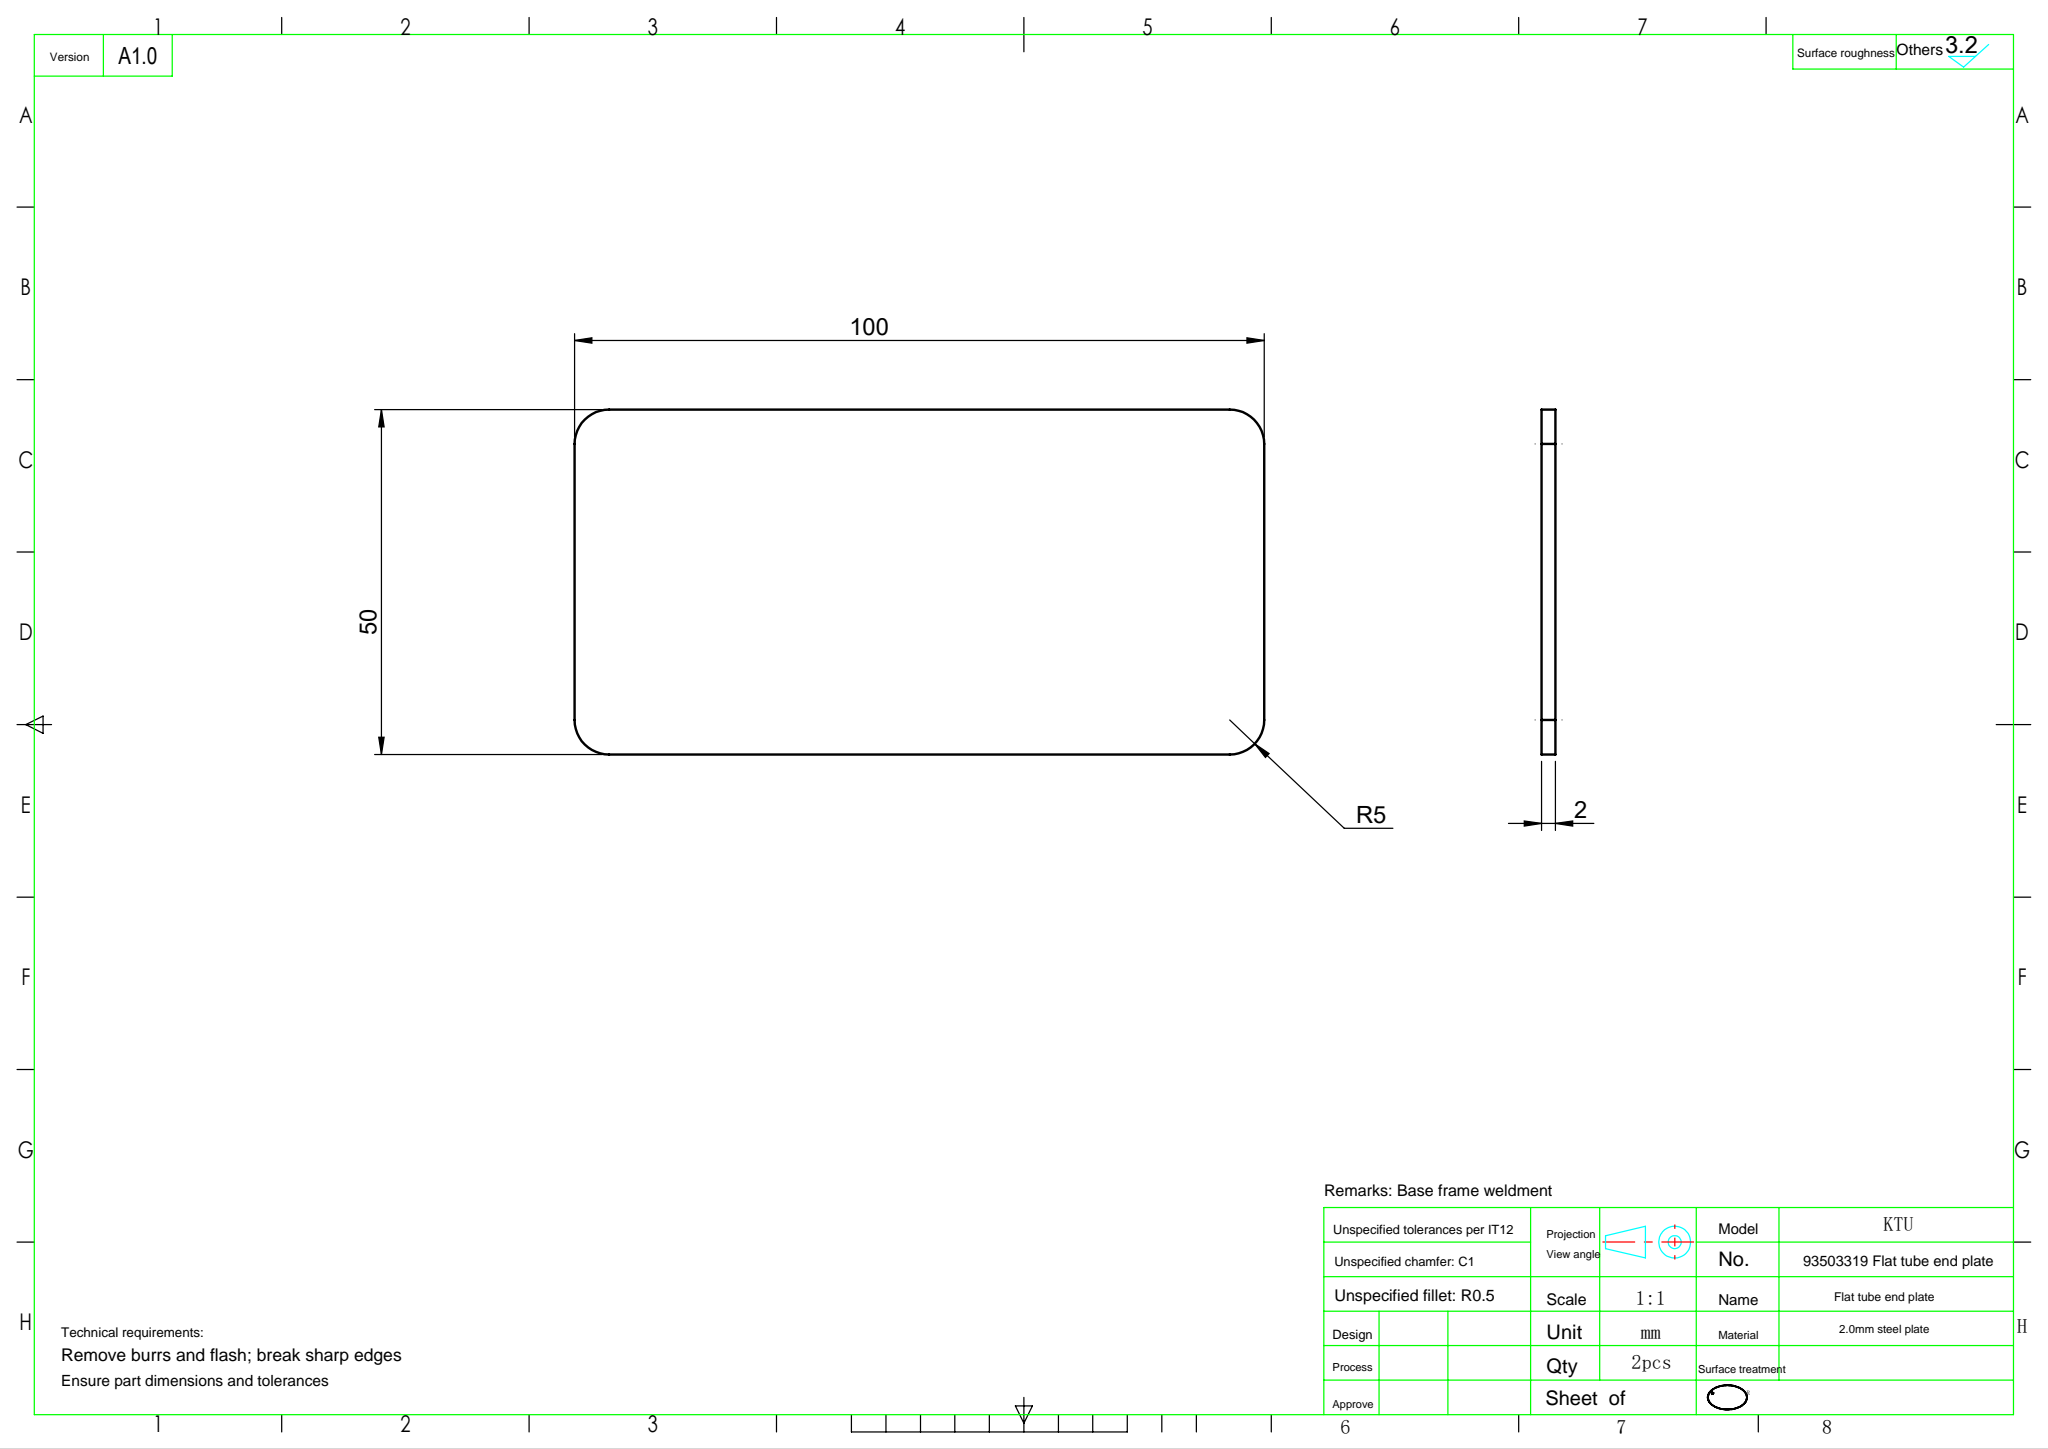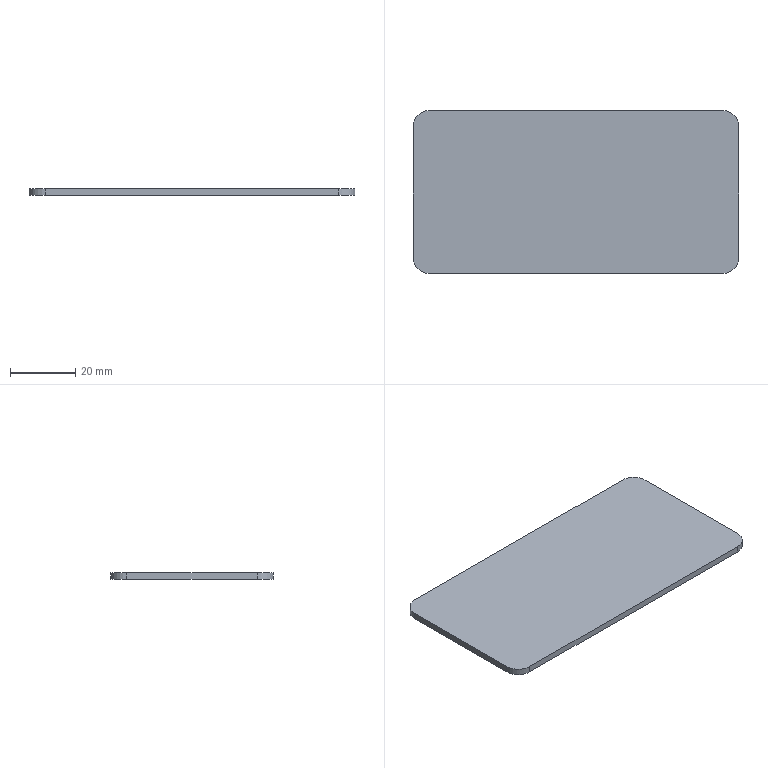Part | SolidWorks | features FlatPattern 1, SMBaseFlange 1, SheetMetal 1 | 1 solid | 10 faces | box 100 x 50 x 2 mm | volume 9957 mm3 | plane 6 | cylinder 4 | commonest cylinder face diameters 10 x4
STEP:
#1=CARTESIAN_POINT('',(45.,-25.,0.));
#2=VERTEX_POINT('',#1);
#3=CARTESIAN_POINT('',(50.,-20.,0.));
#4=VERTEX_POINT('',#3);
#5=CARTESIAN_POINT('',(45.,-20.,0.));
#6=DIRECTION('',(0.,0.,1.));
#7=DIRECTION('',(1.,0.,0.));
#8=AXIS2_PLACEMENT_3D('',#5,#6,#7);
#9=CIRCLE('',#8,5.);
#10=EDGE_CURVE('',#2,#4,#9,.T.);
#11=ORIENTED_EDGE('',*,*,#10,.F.);
#12=CARTESIAN_POINT('',(45.,-25.,-2.));
#13=VERTEX_POINT('',#12);
#14=CARTESIAN_POINT('',(45.,-25.,-2.));
#15=DIRECTION('',(0.,0.,1.));
#16=VECTOR('',#15,1000.);
#17=LINE('',#14,#16);
#18=EDGE_CURVE('',#13,#2,#17,.T.);
#19=ORIENTED_EDGE('',*,*,#18,.F.);
#20=CARTESIAN_POINT('',(50.,-20.,-2.));
#21=VERTEX_POINT('',#20);
#22=CARTESIAN_POINT('',(45.,-20.,-2.));
#23=DIRECTION('',(0.,0.,1.));
#24=DIRECTION('',(1.,0.,0.));
#25=AXIS2_PLACEMENT_3D('',#22,#23,#24);
#26=CIRCLE('',#25,5.);
#27=EDGE_CURVE('',#13,#21,#26,.T.);
#28=ORIENTED_EDGE('',*,*,#27,.T.);
#29=CARTESIAN_POINT('',(50.,-20.,-2.));
#30=DIRECTION('',(0.,0.,1.));
#31=VECTOR('',#30,1000.);
#32=LINE('',#29,#31);
#33=EDGE_CURVE('',#21,#4,#32,.T.);
#34=ORIENTED_EDGE('',*,*,#33,.T.);
#35=EDGE_LOOP('',(#11,#19,#28,#34));
#36=FACE_OUTER_BOUND('',#35,.T.);
#37=CARTESIAN_POINT('',(45.,-20.,-2.));
#38=DIRECTION('',(0.,0.,1.));
#39=DIRECTION('',(1.,0.,0.));
#40=AXIS2_PLACEMENT_3D('',#37,#38,#39);
#41=CYLINDRICAL_SURFACE('',#40,5.);
#42=ADVANCED_FACE('',(#36),#41,.T.);
#43=CARTESIAN_POINT('',(-45.,-25.,0.));
#44=VERTEX_POINT('',#43);
#45=CARTESIAN_POINT('',(-45.,-25.,0.));
#46=DIRECTION('',(1.,0.,0.));
#47=VECTOR('',#46,1000.);
#48=LINE('',#45,#47);
#49=EDGE_CURVE('',#44,#2,#48,.T.);
#50=ORIENTED_EDGE('',*,*,#49,.F.);
#51=CARTESIAN_POINT('',(-45.,-25.,-2.));
#52=VERTEX_POINT('',#51);
#53=CARTESIAN_POINT('',(-45.,-25.,-2.));
#54=DIRECTION('',(0.,0.,1.));
#55=VECTOR('',#54,1000.);
#56=LINE('',#53,#55);
#57=EDGE_CURVE('',#52,#44,#56,.T.);
#58=ORIENTED_EDGE('',*,*,#57,.F.);
#59=CARTESIAN_POINT('',(-45.,-25.,-2.));
#60=DIRECTION('',(1.,0.,0.));
#61=VECTOR('',#60,1000.);
#62=LINE('',#59,#61);
#63=EDGE_CURVE('',#52,#13,#62,.T.);
#64=ORIENTED_EDGE('',*,*,#63,.T.);
#65=ORIENTED_EDGE('',*,*,#18,.T.);
#66=EDGE_LOOP('',(#50,#58,#64,#65));
#67=FACE_OUTER_BOUND('',#66,.T.);
#68=CARTESIAN_POINT('',(-45.,-25.,-2.));
#69=DIRECTION('',(0.,-1.,0.));
#70=DIRECTION('',(0.,0.,-1.));
#71=AXIS2_PLACEMENT_3D('',#68,#69,#70);
#72=PLANE('',#71);
#73=ADVANCED_FACE('',(#67),#72,.T.);
#74=CARTESIAN_POINT('',(-50.,-20.,0.));
#75=VERTEX_POINT('',#74);
#76=CARTESIAN_POINT('',(-45.,-20.,0.));
#77=DIRECTION('',(0.,0.,1.));
#78=DIRECTION('',(-1.,0.,0.));
#79=AXIS2_PLACEMENT_3D('',#76,#77,#78);
#80=CIRCLE('',#79,5.);
#81=EDGE_CURVE('',#75,#44,#80,.T.);
#82=ORIENTED_EDGE('',*,*,#81,.F.);
#83=CARTESIAN_POINT('',(-50.,-20.,-2.));
#84=VERTEX_POINT('',#83);
#85=CARTESIAN_POINT('',(-50.,-20.,-2.));
#86=DIRECTION('',(0.,0.,1.));
#87=VECTOR('',#86,1000.);
#88=LINE('',#85,#87);
#89=EDGE_CURVE('',#84,#75,#88,.T.);
#90=ORIENTED_EDGE('',*,*,#89,.F.);
#91=CARTESIAN_POINT('',(-45.,-20.,-2.));
#92=DIRECTION('',(0.,0.,1.));
#93=DIRECTION('',(-1.,0.,0.));
#94=AXIS2_PLACEMENT_3D('',#91,#92,#93);
#95=CIRCLE('',#94,5.);
#96=EDGE_CURVE('',#84,#52,#95,.T.);
#97=ORIENTED_EDGE('',*,*,#96,.T.);
#98=ORIENTED_EDGE('',*,*,#57,.T.);
#99=EDGE_LOOP('',(#82,#90,#97,#98));
#100=FACE_OUTER_BOUND('',#99,.T.);
#101=CARTESIAN_POINT('',(-45.,-20.,-2.));
#102=DIRECTION('',(0.,0.,1.));
#103=DIRECTION('',(1.,0.,0.));
#104=AXIS2_PLACEMENT_3D('',#101,#102,#103);
#105=CYLINDRICAL_SURFACE('',#104,5.);
#106=ADVANCED_FACE('',(#100),#105,.T.);
#107=CARTESIAN_POINT('',(-50.,20.,0.));
#108=VERTEX_POINT('',#107);
#109=CARTESIAN_POINT('',(-50.,-20.,0.));
#110=DIRECTION('',(0.,-1.,0.));
#111=VECTOR('',#110,1000.);
#112=LINE('',#109,#111);
#113=EDGE_CURVE('',#108,#75,#112,.T.);
#114=ORIENTED_EDGE('',*,*,#113,.F.);
#115=CARTESIAN_POINT('',(-50.,20.,-2.));
#116=VERTEX_POINT('',#115);
#117=CARTESIAN_POINT('',(-50.,20.,-2.));
#118=DIRECTION('',(0.,0.,1.));
#119=VECTOR('',#118,1000.);
#120=LINE('',#117,#119);
#121=EDGE_CURVE('',#116,#108,#120,.T.);
#122=ORIENTED_EDGE('',*,*,#121,.F.);
#123=CARTESIAN_POINT('',(-50.,-20.,-2.));
#124=DIRECTION('',(0.,-1.,0.));
#125=VECTOR('',#124,1000.);
#126=LINE('',#123,#125);
#127=EDGE_CURVE('',#116,#84,#126,.T.);
#128=ORIENTED_EDGE('',*,*,#127,.T.);
#129=ORIENTED_EDGE('',*,*,#89,.T.);
#130=EDGE_LOOP('',(#114,#122,#128,#129));
#131=FACE_OUTER_BOUND('',#130,.T.);
#132=CARTESIAN_POINT('',(-50.,-20.,-2.));
#133=DIRECTION('',(-1.,0.,0.));
#134=DIRECTION('',(0.,0.,1.));
#135=AXIS2_PLACEMENT_3D('',#132,#133,#134);
#136=PLANE('',#135);
#137=ADVANCED_FACE('',(#131),#136,.T.);
#138=CARTESIAN_POINT('',(-45.,25.,0.));
#139=VERTEX_POINT('',#138);
#140=CARTESIAN_POINT('',(-45.,20.,0.));
#141=DIRECTION('',(0.,0.,1.));
#142=DIRECTION('',(-1.,0.,0.));
#143=AXIS2_PLACEMENT_3D('',#140,#141,#142);
#144=CIRCLE('',#143,5.);
#145=EDGE_CURVE('',#139,#108,#144,.T.);
#146=ORIENTED_EDGE('',*,*,#145,.F.);
#147=CARTESIAN_POINT('',(-45.,25.,-2.));
#148=VERTEX_POINT('',#147);
#149=CARTESIAN_POINT('',(-45.,25.,-2.));
#150=DIRECTION('',(0.,0.,1.));
#151=VECTOR('',#150,1000.);
#152=LINE('',#149,#151);
#153=EDGE_CURVE('',#148,#139,#152,.T.);
#154=ORIENTED_EDGE('',*,*,#153,.F.);
#155=CARTESIAN_POINT('',(-45.,20.,-2.));
#156=DIRECTION('',(0.,0.,1.));
#157=DIRECTION('',(-1.,0.,0.));
#158=AXIS2_PLACEMENT_3D('',#155,#156,#157);
#159=CIRCLE('',#158,5.);
#160=EDGE_CURVE('',#148,#116,#159,.T.);
#161=ORIENTED_EDGE('',*,*,#160,.T.);
#162=ORIENTED_EDGE('',*,*,#121,.T.);
#163=EDGE_LOOP('',(#146,#154,#161,#162));
#164=FACE_OUTER_BOUND('',#163,.T.);
#165=CARTESIAN_POINT('',(-45.,20.,-2.));
#166=DIRECTION('',(0.,0.,1.));
#167=DIRECTION('',(1.,0.,0.));
#168=AXIS2_PLACEMENT_3D('',#165,#166,#167);
#169=CYLINDRICAL_SURFACE('',#168,5.);
#170=ADVANCED_FACE('',(#164),#169,.T.);
#171=CARTESIAN_POINT('',(45.,25.,0.));
#172=VERTEX_POINT('',#171);
#173=CARTESIAN_POINT('',(-45.,25.,0.));
#174=DIRECTION('',(-1.,0.,0.));
#175=VECTOR('',#174,1000.);
#176=LINE('',#173,#175);
#177=EDGE_CURVE('',#172,#139,#176,.T.);
#178=ORIENTED_EDGE('',*,*,#177,.F.);
#179=CARTESIAN_POINT('',(45.,25.,-2.));
#180=VERTEX_POINT('',#179);
#181=CARTESIAN_POINT('',(45.,25.,-2.));
#182=DIRECTION('',(0.,0.,1.));
#183=VECTOR('',#182,1000.);
#184=LINE('',#181,#183);
#185=EDGE_CURVE('',#180,#172,#184,.T.);
#186=ORIENTED_EDGE('',*,*,#185,.F.);
#187=CARTESIAN_POINT('',(-45.,25.,-2.));
#188=DIRECTION('',(-1.,0.,0.));
#189=VECTOR('',#188,1000.);
#190=LINE('',#187,#189);
#191=EDGE_CURVE('',#180,#148,#190,.T.);
#192=ORIENTED_EDGE('',*,*,#191,.T.);
#193=ORIENTED_EDGE('',*,*,#153,.T.);
#194=EDGE_LOOP('',(#178,#186,#192,#193));
#195=FACE_OUTER_BOUND('',#194,.T.);
#196=CARTESIAN_POINT('',(-45.,25.,-2.));
#197=DIRECTION('',(0.,1.,0.));
#198=DIRECTION('',(0.,0.,1.));
#199=AXIS2_PLACEMENT_3D('',#196,#197,#198);
#200=PLANE('',#199);
#201=ADVANCED_FACE('',(#195),#200,.T.);
#202=CARTESIAN_POINT('',(50.,20.,0.));
#203=VERTEX_POINT('',#202);
#204=CARTESIAN_POINT('',(45.,20.,0.));
#205=DIRECTION('',(0.,0.,1.));
#206=DIRECTION('',(-1.,0.,0.));
#207=AXIS2_PLACEMENT_3D('',#204,#205,#206);
#208=CIRCLE('',#207,5.);
#209=EDGE_CURVE('',#203,#172,#208,.T.);
#210=ORIENTED_EDGE('',*,*,#209,.F.);
#211=CARTESIAN_POINT('',(50.,20.,-2.));
#212=VERTEX_POINT('',#211);
#213=CARTESIAN_POINT('',(50.,20.,-2.));
#214=DIRECTION('',(0.,0.,1.));
#215=VECTOR('',#214,1000.);
#216=LINE('',#213,#215);
#217=EDGE_CURVE('',#212,#203,#216,.T.);
#218=ORIENTED_EDGE('',*,*,#217,.F.);
#219=CARTESIAN_POINT('',(45.,20.,-2.));
#220=DIRECTION('',(0.,0.,1.));
#221=DIRECTION('',(-1.,0.,0.));
#222=AXIS2_PLACEMENT_3D('',#219,#220,#221);
#223=CIRCLE('',#222,5.);
#224=EDGE_CURVE('',#212,#180,#223,.T.);
#225=ORIENTED_EDGE('',*,*,#224,.T.);
#226=ORIENTED_EDGE('',*,*,#185,.T.);
#227=EDGE_LOOP('',(#210,#218,#225,#226));
#228=FACE_OUTER_BOUND('',#227,.T.);
#229=CARTESIAN_POINT('',(45.,20.,-2.));
#230=DIRECTION('',(0.,0.,1.));
#231=DIRECTION('',(1.,0.,0.));
#232=AXIS2_PLACEMENT_3D('',#229,#230,#231);
#233=CYLINDRICAL_SURFACE('',#232,5.);
#234=ADVANCED_FACE('',(#228),#233,.T.);
#235=CARTESIAN_POINT('',(50.,-20.,0.));
#236=DIRECTION('',(0.,1.,0.));
#237=VECTOR('',#236,1000.);
#238=LINE('',#235,#237);
#239=EDGE_CURVE('',#4,#203,#238,.T.);
#240=ORIENTED_EDGE('',*,*,#239,.F.);
#241=ORIENTED_EDGE('',*,*,#33,.F.);
#242=CARTESIAN_POINT('',(50.,-20.,-2.));
#243=DIRECTION('',(0.,1.,0.));
#244=VECTOR('',#243,1000.);
#245=LINE('',#242,#244);
#246=EDGE_CURVE('',#21,#212,#245,.T.);
#247=ORIENTED_EDGE('',*,*,#246,.T.);
#248=ORIENTED_EDGE('',*,*,#217,.T.);
#249=EDGE_LOOP('',(#240,#241,#247,#248));
#250=FACE_OUTER_BOUND('',#249,.T.);
#251=CARTESIAN_POINT('',(50.,-20.,-2.));
#252=DIRECTION('',(1.,0.,0.));
#253=DIRECTION('',(0.,0.,-1.));
#254=AXIS2_PLACEMENT_3D('',#251,#252,#253);
#255=PLANE('',#254);
#256=ADVANCED_FACE('',(#250),#255,.T.);
#257=ORIENTED_EDGE('',*,*,#27,.F.);
#258=ORIENTED_EDGE('',*,*,#63,.F.);
#259=ORIENTED_EDGE('',*,*,#96,.F.);
#260=ORIENTED_EDGE('',*,*,#127,.F.);
#261=ORIENTED_EDGE('',*,*,#160,.F.);
#262=ORIENTED_EDGE('',*,*,#191,.F.);
#263=ORIENTED_EDGE('',*,*,#224,.F.);
#264=ORIENTED_EDGE('',*,*,#246,.F.);
#265=EDGE_LOOP('',(#257,#258,#259,#260,#261,#262,#263,#264));
#266=FACE_OUTER_BOUND('',#265,.T.);
#267=CARTESIAN_POINT('',(45.,-20.,-2.));
#268=DIRECTION('',(0.,0.,1.));
#269=DIRECTION('',(1.,0.,0.));
#270=AXIS2_PLACEMENT_3D('',#267,#268,#269);
#271=PLANE('',#270);
#272=ADVANCED_FACE('',(#266),#271,.F.);
#273=ORIENTED_EDGE('',*,*,#10,.T.);
#274=ORIENTED_EDGE('',*,*,#239,.T.);
#275=ORIENTED_EDGE('',*,*,#209,.T.);
#276=ORIENTED_EDGE('',*,*,#177,.T.);
#277=ORIENTED_EDGE('',*,*,#145,.T.);
#278=ORIENTED_EDGE('',*,*,#113,.T.);
#279=ORIENTED_EDGE('',*,*,#81,.T.);
#280=ORIENTED_EDGE('',*,*,#49,.T.);
#281=EDGE_LOOP('',(#273,#274,#275,#276,#277,#278,#279,#280));
#282=FACE_OUTER_BOUND('',#281,.T.);
#283=CARTESIAN_POINT('',(45.,-20.,0.));
#284=DIRECTION('',(0.,0.,1.));
#285=DIRECTION('',(1.,0.,0.));
#286=AXIS2_PLACEMENT_3D('',#283,#284,#285);
#287=PLANE('',#286);
#288=ADVANCED_FACE('',(#282),#287,.T.);
#289=CLOSED_SHELL('',(#42,#73,#106,#137,#170,#201,#234,#256,#272,#288));
#290=MANIFOLD_SOLID_BREP('',#289);
#291=CARTESIAN_POINT('',(0.,0.,0.));
#292=DIRECTION('',(0.,0.,1.));
#293=DIRECTION('',(1.,0.,0.));
#294=AXIS2_PLACEMENT_3D('',#291,#292,#293);
#295=(LENGTH_UNIT()NAMED_UNIT(*)SI_UNIT(.MILLI.,.METRE.));
#296=UNCERTAINTY_MEASURE_WITH_UNIT(LENGTH_MEASURE(0.00001),#295,'','');
#297=(NAMED_UNIT(*)PLANE_ANGLE_UNIT()SI_UNIT($,.RADIAN.));
#298=(NAMED_UNIT(*)SI_UNIT($,.STERADIAN.)SOLID_ANGLE_UNIT());
#299=(GEOMETRIC_REPRESENTATION_CONTEXT(3)GLOBAL_UNCERTAINTY_ASSIGNED_CONTEXT((#296))GLOBAL_UNIT_ASSIGNED_CONTEXT((#295,#297,#298))REPRESENTATION_CONTEXT('',''));
#300=ADVANCED_BREP_SHAPE_REPRESENTATION('',(#290,#294),#299);